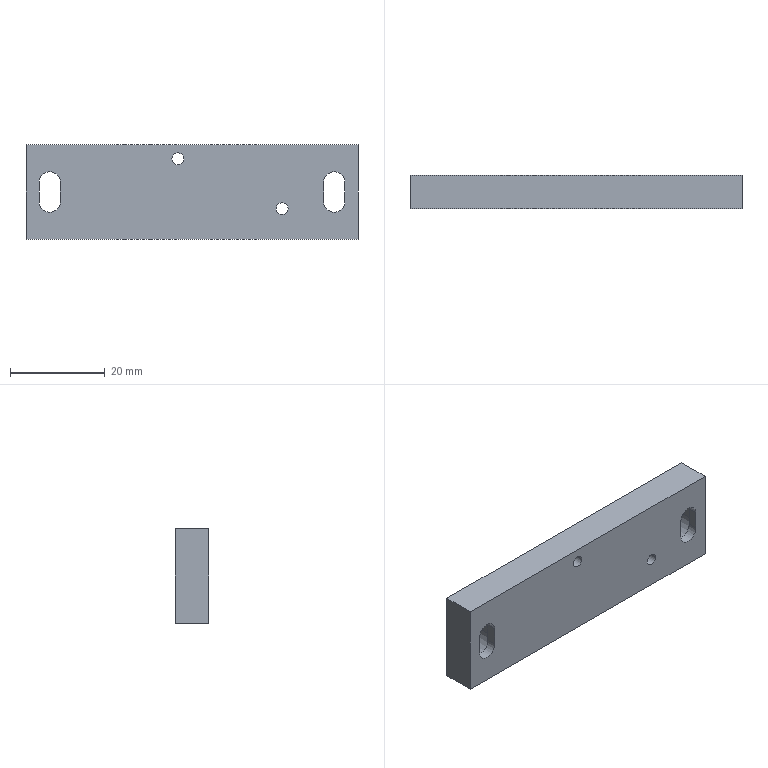Part | Creo | 1 solid | 32 faces | box 70 x 7 x 20 mm | volume 8772 mm3 | plane 16 | cylinder 12 | cone 4 | commonest cylinder face diameters 2.5 x4 4.5 x4 8 x4
STEP:
#1=CARTESIAN_POINT('',(-13.75,343.995,-332.));
#2=VERTEX_POINT('',#1);
#3=CARTESIAN_POINT('',(-83.75,343.995,-332.));
#4=VERTEX_POINT('',#3);
#5=CARTESIAN_POINT('',(-13.75,343.995,-332.));
#6=DIRECTION('',(-1.,0.,0.));
#7=VECTOR('',#6,70.);
#8=LINE('',#5,#7);
#9=EDGE_CURVE('',#2,#4,#8,.T.);
#10=ORIENTED_EDGE('',*,*,#9,.F.);
#11=CARTESIAN_POINT('',(-13.75,343.995,-352.));
#12=VERTEX_POINT('',#11);
#13=CARTESIAN_POINT('',(-13.75,343.995,-352.));
#14=DIRECTION('',(0.,0.,1.));
#15=VECTOR('',#14,20.);
#16=LINE('',#13,#15);
#17=EDGE_CURVE('',#12,#2,#16,.T.);
#18=ORIENTED_EDGE('',*,*,#17,.F.);
#19=CARTESIAN_POINT('',(-83.75,343.995,-352.));
#20=VERTEX_POINT('',#19);
#21=CARTESIAN_POINT('',(-83.75,343.995,-352.));
#22=DIRECTION('',(1.,0.,0.));
#23=VECTOR('',#22,70.);
#24=LINE('',#21,#23);
#25=EDGE_CURVE('',#20,#12,#24,.T.);
#26=ORIENTED_EDGE('',*,*,#25,.F.);
#27=CARTESIAN_POINT('',(-83.75,343.995,-332.));
#28=DIRECTION('',(0.,0.,-1.));
#29=VECTOR('',#28,20.);
#30=LINE('',#27,#29);
#31=EDGE_CURVE('',#4,#20,#30,.T.);
#32=ORIENTED_EDGE('',*,*,#31,.F.);
#33=EDGE_LOOP('',(#10,#18,#26,#32));
#34=FACE_OUTER_BOUND('',#33,.F.);
#35=CARTESIAN_POINT('',(-16.5,343.995,-344.));
#36=VERTEX_POINT('',#35);
#37=CARTESIAN_POINT('',(-16.5,343.995,-340.));
#38=VERTEX_POINT('',#37);
#39=CARTESIAN_POINT('',(-16.5,343.995,-344.));
#40=DIRECTION('',(0.,0.,1.));
#41=VECTOR('',#40,4.);
#42=LINE('',#39,#41);
#43=EDGE_CURVE('',#36,#38,#42,.T.);
#44=ORIENTED_EDGE('',*,*,#43,.T.);
#45=CARTESIAN_POINT('',(-21.,343.995,-340.));
#46=VERTEX_POINT('',#45);
#47=CARTESIAN_POINT('',(-18.75,343.995,-340.));
#48=DIRECTION('',(0.,1.,0.));
#49=DIRECTION('',(-1.,0.,0.));
#50=AXIS2_PLACEMENT_3D('',#47,#48,#49);
#51=CIRCLE('',#50,2.25);
#52=EDGE_CURVE('',#46,#38,#51,.T.);
#53=ORIENTED_EDGE('',*,*,#52,.F.);
#54=CARTESIAN_POINT('',(-21.,343.995,-344.));
#55=VERTEX_POINT('',#54);
#56=CARTESIAN_POINT('',(-21.,343.995,-340.));
#57=DIRECTION('',(0.,0.,-1.));
#58=VECTOR('',#57,4.);
#59=LINE('',#56,#58);
#60=EDGE_CURVE('',#46,#55,#59,.T.);
#61=ORIENTED_EDGE('',*,*,#60,.T.);
#62=CARTESIAN_POINT('',(-18.75,343.995,-344.));
#63=DIRECTION('',(0.,1.,0.));
#64=DIRECTION('',(1.,0.,0.));
#65=AXIS2_PLACEMENT_3D('',#62,#63,#64);
#66=CIRCLE('',#65,2.25);
#67=EDGE_CURVE('',#36,#55,#66,.T.);
#68=ORIENTED_EDGE('',*,*,#67,.F.);
#69=EDGE_LOOP('',(#44,#53,#61,#68));
#70=FACE_BOUND('',#69,.F.);
#71=CARTESIAN_POINT('',(-76.5,343.995,-344.));
#72=VERTEX_POINT('',#71);
#73=CARTESIAN_POINT('',(-81.,343.995,-344.));
#74=VERTEX_POINT('',#73);
#75=CARTESIAN_POINT('',(-78.75,343.995,-344.));
#76=DIRECTION('',(0.,1.,0.));
#77=DIRECTION('',(1.,0.,0.));
#78=AXIS2_PLACEMENT_3D('',#75,#76,#77);
#79=CIRCLE('',#78,2.25);
#80=EDGE_CURVE('',#72,#74,#79,.T.);
#81=ORIENTED_EDGE('',*,*,#80,.F.);
#82=CARTESIAN_POINT('',(-76.5,343.995,-340.));
#83=VERTEX_POINT('',#82);
#84=CARTESIAN_POINT('',(-76.5,343.995,-344.));
#85=DIRECTION('',(0.,0.,1.));
#86=VECTOR('',#85,4.);
#87=LINE('',#84,#86);
#88=EDGE_CURVE('',#72,#83,#87,.T.);
#89=ORIENTED_EDGE('',*,*,#88,.T.);
#90=CARTESIAN_POINT('',(-81.,343.995,-340.));
#91=VERTEX_POINT('',#90);
#92=CARTESIAN_POINT('',(-78.75,343.995,-340.));
#93=DIRECTION('',(0.,1.,0.));
#94=DIRECTION('',(-1.,0.,0.));
#95=AXIS2_PLACEMENT_3D('',#92,#93,#94);
#96=CIRCLE('',#95,2.25);
#97=EDGE_CURVE('',#91,#83,#96,.T.);
#98=ORIENTED_EDGE('',*,*,#97,.F.);
#99=CARTESIAN_POINT('',(-81.,343.995,-340.));
#100=DIRECTION('',(0.,0.,-1.));
#101=VECTOR('',#100,4.);
#102=LINE('',#99,#101);
#103=EDGE_CURVE('',#91,#74,#102,.T.);
#104=ORIENTED_EDGE('',*,*,#103,.T.);
#105=EDGE_LOOP('',(#81,#89,#98,#104));
#106=FACE_BOUND('',#105,.F.);
#107=CARTESIAN_POINT('',(-53.,343.995,-335.));
#108=VERTEX_POINT('',#107);
#109=CARTESIAN_POINT('',(-50.5,343.995,-335.));
#110=VERTEX_POINT('',#109);
#111=CARTESIAN_POINT('',(-51.75,343.995,-335.));
#112=DIRECTION('',(0.,1.,0.));
#113=DIRECTION('',(-1.,0.,0.));
#114=AXIS2_PLACEMENT_3D('',#111,#112,#113);
#115=CIRCLE('',#114,1.25);
#116=EDGE_CURVE('',#108,#110,#115,.T.);
#117=ORIENTED_EDGE('',*,*,#116,.F.);
#118=CARTESIAN_POINT('',(-51.75,343.995,-335.));
#119=DIRECTION('',(0.,1.,0.));
#120=DIRECTION('',(1.,0.,0.));
#121=AXIS2_PLACEMENT_3D('',#118,#119,#120);
#122=CIRCLE('',#121,1.25);
#123=EDGE_CURVE('',#110,#108,#122,.T.);
#124=ORIENTED_EDGE('',*,*,#123,.F.);
#125=EDGE_LOOP('',(#117,#124));
#126=FACE_BOUND('',#125,.F.);
#127=CARTESIAN_POINT('',(-31.,343.995,-345.5));
#128=VERTEX_POINT('',#127);
#129=CARTESIAN_POINT('',(-28.5,343.995,-345.5));
#130=VERTEX_POINT('',#129);
#131=CARTESIAN_POINT('',(-29.75,343.995,-345.5));
#132=DIRECTION('',(0.,1.,0.));
#133=DIRECTION('',(-1.,0.,0.));
#134=AXIS2_PLACEMENT_3D('',#131,#132,#133);
#135=CIRCLE('',#134,1.25);
#136=EDGE_CURVE('',#128,#130,#135,.T.);
#137=ORIENTED_EDGE('',*,*,#136,.F.);
#138=CARTESIAN_POINT('',(-29.75,343.995,-345.5));
#139=DIRECTION('',(0.,1.,0.));
#140=DIRECTION('',(1.,0.,0.));
#141=AXIS2_PLACEMENT_3D('',#138,#139,#140);
#142=CIRCLE('',#141,1.25);
#143=EDGE_CURVE('',#130,#128,#142,.T.);
#144=ORIENTED_EDGE('',*,*,#143,.F.);
#145=EDGE_LOOP('',(#137,#144));
#146=FACE_BOUND('',#145,.F.);
#147=CARTESIAN_POINT('',(-48.75,343.995,-342.));
#148=DIRECTION('',(0.,1.,0.));
#149=DIRECTION('',(1.,0.,0.));
#150=AXIS2_PLACEMENT_3D('',#147,#148,#149);
#151=PLANE('',#150);
#152=ADVANCED_FACE('',(#34,#70,#106,#126,#146),#151,.F.);
#153=CARTESIAN_POINT('',(-13.75,350.995,-332.));
#154=VERTEX_POINT('',#153);
#155=CARTESIAN_POINT('',(-13.75,350.995,-332.));
#156=DIRECTION('',(0.,-1.,0.));
#157=VECTOR('',#156,7.);
#158=LINE('',#155,#157);
#159=EDGE_CURVE('',#154,#2,#158,.T.);
#160=ORIENTED_EDGE('',*,*,#159,.T.);
#161=ORIENTED_EDGE('',*,*,#9,.T.);
#162=CARTESIAN_POINT('',(-83.75,350.995,-332.));
#163=VERTEX_POINT('',#162);
#164=CARTESIAN_POINT('',(-83.75,350.995,-332.));
#165=DIRECTION('',(0.,-1.,0.));
#166=VECTOR('',#165,7.);
#167=LINE('',#164,#166);
#168=EDGE_CURVE('',#163,#4,#167,.T.);
#169=ORIENTED_EDGE('',*,*,#168,.F.);
#170=CARTESIAN_POINT('',(-13.75,350.995,-332.));
#171=DIRECTION('',(-1.,0.,0.));
#172=VECTOR('',#171,70.);
#173=LINE('',#170,#172);
#174=EDGE_CURVE('',#154,#163,#173,.T.);
#175=ORIENTED_EDGE('',*,*,#174,.F.);
#176=EDGE_LOOP('',(#160,#161,#169,#175));
#177=FACE_OUTER_BOUND('',#176,.F.);
#178=CARTESIAN_POINT('',(-83.75,343.995,-332.));
#179=DIRECTION('',(0.,0.,1.));
#180=DIRECTION('',(-1.,0.,0.));
#181=AXIS2_PLACEMENT_3D('',#178,#179,#180);
#182=PLANE('',#181);
#183=ADVANCED_FACE('',(#177),#182,.T.);
#184=CARTESIAN_POINT('',(-13.75,350.995,-352.));
#185=VERTEX_POINT('',#184);
#186=CARTESIAN_POINT('',(-13.75,350.995,-352.));
#187=DIRECTION('',(0.,-1.,0.));
#188=VECTOR('',#187,7.);
#189=LINE('',#186,#188);
#190=EDGE_CURVE('',#185,#12,#189,.T.);
#191=ORIENTED_EDGE('',*,*,#190,.T.);
#192=ORIENTED_EDGE('',*,*,#17,.T.);
#193=ORIENTED_EDGE('',*,*,#159,.F.);
#194=CARTESIAN_POINT('',(-13.75,350.995,-352.));
#195=DIRECTION('',(0.,0.,1.));
#196=VECTOR('',#195,20.);
#197=LINE('',#194,#196);
#198=EDGE_CURVE('',#185,#154,#197,.T.);
#199=ORIENTED_EDGE('',*,*,#198,.F.);
#200=EDGE_LOOP('',(#191,#192,#193,#199));
#201=FACE_OUTER_BOUND('',#200,.F.);
#202=CARTESIAN_POINT('',(-13.75,343.995,-332.));
#203=DIRECTION('',(1.,0.,0.));
#204=DIRECTION('',(0.,0.,1.));
#205=AXIS2_PLACEMENT_3D('',#202,#203,#204);
#206=PLANE('',#205);
#207=ADVANCED_FACE('',(#201),#206,.T.);
#208=CARTESIAN_POINT('',(-83.75,350.995,-352.));
#209=VERTEX_POINT('',#208);
#210=CARTESIAN_POINT('',(-83.75,350.995,-352.));
#211=DIRECTION('',(0.,-1.,0.));
#212=VECTOR('',#211,7.);
#213=LINE('',#210,#212);
#214=EDGE_CURVE('',#209,#20,#213,.T.);
#215=ORIENTED_EDGE('',*,*,#214,.T.);
#216=ORIENTED_EDGE('',*,*,#25,.T.);
#217=ORIENTED_EDGE('',*,*,#190,.F.);
#218=CARTESIAN_POINT('',(-83.75,350.995,-352.));
#219=DIRECTION('',(1.,0.,0.));
#220=VECTOR('',#219,70.);
#221=LINE('',#218,#220);
#222=EDGE_CURVE('',#209,#185,#221,.T.);
#223=ORIENTED_EDGE('',*,*,#222,.F.);
#224=EDGE_LOOP('',(#215,#216,#217,#223));
#225=FACE_OUTER_BOUND('',#224,.F.);
#226=CARTESIAN_POINT('',(-13.75,343.995,-352.));
#227=DIRECTION('',(0.,0.,-1.));
#228=DIRECTION('',(1.,0.,0.));
#229=AXIS2_PLACEMENT_3D('',#226,#227,#228);
#230=PLANE('',#229);
#231=ADVANCED_FACE('',(#225),#230,.T.);
#232=ORIENTED_EDGE('',*,*,#168,.T.);
#233=ORIENTED_EDGE('',*,*,#31,.T.);
#234=ORIENTED_EDGE('',*,*,#214,.F.);
#235=CARTESIAN_POINT('',(-83.75,350.995,-332.));
#236=DIRECTION('',(0.,0.,-1.));
#237=VECTOR('',#236,20.);
#238=LINE('',#235,#237);
#239=EDGE_CURVE('',#163,#209,#238,.T.);
#240=ORIENTED_EDGE('',*,*,#239,.F.);
#241=EDGE_LOOP('',(#232,#233,#234,#240));
#242=FACE_OUTER_BOUND('',#241,.F.);
#243=CARTESIAN_POINT('',(-83.75,343.995,-352.));
#244=DIRECTION('',(-1.,0.,0.));
#245=DIRECTION('',(0.,0.,-1.));
#246=AXIS2_PLACEMENT_3D('',#243,#244,#245);
#247=PLANE('',#246);
#248=ADVANCED_FACE('',(#242),#247,.T.);
#249=ORIENTED_EDGE('',*,*,#222,.T.);
#250=ORIENTED_EDGE('',*,*,#198,.T.);
#251=ORIENTED_EDGE('',*,*,#174,.T.);
#252=ORIENTED_EDGE('',*,*,#239,.T.);
#253=EDGE_LOOP('',(#249,#250,#251,#252));
#254=FACE_OUTER_BOUND('',#253,.F.);
#255=CARTESIAN_POINT('',(-22.75,350.995,-340.));
#256=VERTEX_POINT('',#255);
#257=CARTESIAN_POINT('',(-22.75,350.995,-344.));
#258=VERTEX_POINT('',#257);
#259=CARTESIAN_POINT('',(-22.75,350.995,-340.));
#260=DIRECTION('',(0.,0.,-1.));
#261=VECTOR('',#260,4.);
#262=LINE('',#259,#261);
#263=EDGE_CURVE('',#256,#258,#262,.T.);
#264=ORIENTED_EDGE('',*,*,#263,.F.);
#265=CARTESIAN_POINT('',(-14.75,350.995,-340.));
#266=VERTEX_POINT('',#265);
#267=CARTESIAN_POINT('',(-18.75,350.995,-340.));
#268=DIRECTION('',(0.,-1.,0.));
#269=DIRECTION('',(1.,0.,0.));
#270=AXIS2_PLACEMENT_3D('',#267,#268,#269);
#271=CIRCLE('',#270,4.);
#272=EDGE_CURVE('',#266,#256,#271,.T.);
#273=ORIENTED_EDGE('',*,*,#272,.F.);
#274=CARTESIAN_POINT('',(-14.75,350.995,-344.));
#275=VERTEX_POINT('',#274);
#276=CARTESIAN_POINT('',(-14.75,350.995,-344.));
#277=DIRECTION('',(0.,0.,1.));
#278=VECTOR('',#277,4.);
#279=LINE('',#276,#278);
#280=EDGE_CURVE('',#275,#266,#279,.T.);
#281=ORIENTED_EDGE('',*,*,#280,.F.);
#282=CARTESIAN_POINT('',(-18.75,350.995,-344.));
#283=DIRECTION('',(0.,-1.,0.));
#284=DIRECTION('',(-1.,0.,0.));
#285=AXIS2_PLACEMENT_3D('',#282,#283,#284);
#286=CIRCLE('',#285,4.);
#287=EDGE_CURVE('',#258,#275,#286,.T.);
#288=ORIENTED_EDGE('',*,*,#287,.F.);
#289=EDGE_LOOP('',(#264,#273,#281,#288));
#290=FACE_BOUND('',#289,.F.);
#291=CARTESIAN_POINT('',(-74.75,350.995,-340.));
#292=VERTEX_POINT('',#291);
#293=CARTESIAN_POINT('',(-82.75,350.995,-340.));
#294=VERTEX_POINT('',#293);
#295=CARTESIAN_POINT('',(-78.75,350.995,-340.));
#296=DIRECTION('',(0.,-1.,0.));
#297=DIRECTION('',(1.,0.,0.));
#298=AXIS2_PLACEMENT_3D('',#295,#296,#297);
#299=CIRCLE('',#298,4.);
#300=EDGE_CURVE('',#292,#294,#299,.T.);
#301=ORIENTED_EDGE('',*,*,#300,.F.);
#302=CARTESIAN_POINT('',(-74.75,350.995,-344.));
#303=VERTEX_POINT('',#302);
#304=CARTESIAN_POINT('',(-74.75,350.995,-344.));
#305=DIRECTION('',(0.,0.,1.));
#306=VECTOR('',#305,4.);
#307=LINE('',#304,#306);
#308=EDGE_CURVE('',#303,#292,#307,.T.);
#309=ORIENTED_EDGE('',*,*,#308,.F.);
#310=CARTESIAN_POINT('',(-82.75,350.995,-344.));
#311=VERTEX_POINT('',#310);
#312=CARTESIAN_POINT('',(-78.75,350.995,-344.));
#313=DIRECTION('',(0.,-1.,0.));
#314=DIRECTION('',(-1.,0.,0.));
#315=AXIS2_PLACEMENT_3D('',#312,#313,#314);
#316=CIRCLE('',#315,4.);
#317=EDGE_CURVE('',#311,#303,#316,.T.);
#318=ORIENTED_EDGE('',*,*,#317,.F.);
#319=CARTESIAN_POINT('',(-82.75,350.995,-340.));
#320=DIRECTION('',(0.,0.,-1.));
#321=VECTOR('',#320,4.);
#322=LINE('',#319,#321);
#323=EDGE_CURVE('',#294,#311,#322,.T.);
#324=ORIENTED_EDGE('',*,*,#323,.F.);
#325=EDGE_LOOP('',(#301,#309,#318,#324));
#326=FACE_BOUND('',#325,.F.);
#327=CARTESIAN_POINT('',(-50.188,350.995,-335.));
#328=VERTEX_POINT('',#327);
#329=CARTESIAN_POINT('',(-53.312,350.995,-335.));
#330=VERTEX_POINT('',#329);
#331=CARTESIAN_POINT('',(-51.75,350.995,-335.));
#332=DIRECTION('',(0.,-1.,0.));
#333=DIRECTION('',(1.,0.,0.));
#334=AXIS2_PLACEMENT_3D('',#331,#332,#333);
#335=CIRCLE('',#334,1.562);
#336=EDGE_CURVE('',#328,#330,#335,.T.);
#337=ORIENTED_EDGE('',*,*,#336,.F.);
#338=CARTESIAN_POINT('',(-51.75,350.995,-335.));
#339=DIRECTION('',(0.,-1.,0.));
#340=DIRECTION('',(-1.,0.,0.));
#341=AXIS2_PLACEMENT_3D('',#338,#339,#340);
#342=CIRCLE('',#341,1.562);
#343=EDGE_CURVE('',#330,#328,#342,.T.);
#344=ORIENTED_EDGE('',*,*,#343,.F.);
#345=EDGE_LOOP('',(#337,#344));
#346=FACE_BOUND('',#345,.F.);
#347=CARTESIAN_POINT('',(-28.188,350.995,-345.5));
#348=VERTEX_POINT('',#347);
#349=CARTESIAN_POINT('',(-31.312,350.995,-345.5));
#350=VERTEX_POINT('',#349);
#351=CARTESIAN_POINT('',(-29.75,350.995,-345.5));
#352=DIRECTION('',(0.,-1.,0.));
#353=DIRECTION('',(1.,0.,0.));
#354=AXIS2_PLACEMENT_3D('',#351,#352,#353);
#355=CIRCLE('',#354,1.562);
#356=EDGE_CURVE('',#348,#350,#355,.T.);
#357=ORIENTED_EDGE('',*,*,#356,.F.);
#358=CARTESIAN_POINT('',(-29.75,350.995,-345.5));
#359=DIRECTION('',(0.,-1.,0.));
#360=DIRECTION('',(-1.,0.,0.));
#361=AXIS2_PLACEMENT_3D('',#358,#359,#360);
#362=CIRCLE('',#361,1.562);
#363=EDGE_CURVE('',#350,#348,#362,.T.);
#364=ORIENTED_EDGE('',*,*,#363,.F.);
#365=EDGE_LOOP('',(#357,#364));
#366=FACE_BOUND('',#365,.F.);
#367=CARTESIAN_POINT('',(-48.75,350.995,-342.));
#368=DIRECTION('',(0.,1.,0.));
#369=DIRECTION('',(1.,0.,0.));
#370=AXIS2_PLACEMENT_3D('',#367,#368,#369);
#371=PLANE('',#370);
#372=ADVANCED_FACE('',(#254,#290,#326,#346,#366),#371,.T.);
#373=CARTESIAN_POINT('',(-22.75,345.995,-340.));
#374=VERTEX_POINT('',#373);
#375=CARTESIAN_POINT('',(-22.75,345.995,-340.));
#376=DIRECTION('',(0.,1.,0.));
#377=VECTOR('',#376,5.);
#378=LINE('',#375,#377);
#379=EDGE_CURVE('',#374,#256,#378,.T.);
#380=ORIENTED_EDGE('',*,*,#379,.T.);
#381=ORIENTED_EDGE('',*,*,#263,.T.);
#382=CARTESIAN_POINT('',(-22.75,345.995,-344.));
#383=VERTEX_POINT('',#382);
#384=CARTESIAN_POINT('',(-22.75,350.995,-344.));
#385=DIRECTION('',(0.,-1.,0.));
#386=VECTOR('',#385,5.);
#387=LINE('',#384,#386);
#388=EDGE_CURVE('',#258,#383,#387,.T.);
#389=ORIENTED_EDGE('',*,*,#388,.T.);
#390=CARTESIAN_POINT('',(-22.75,345.995,-340.));
#391=DIRECTION('',(0.,0.,-1.));
#392=VECTOR('',#391,4.);
#393=LINE('',#390,#392);
#394=EDGE_CURVE('',#374,#383,#393,.T.);
#395=ORIENTED_EDGE('',*,*,#394,.F.);
#396=EDGE_LOOP('',(#380,#381,#389,#395));
#397=FACE_OUTER_BOUND('',#396,.F.);
#398=CARTESIAN_POINT('',(-22.75,350.995,-344.));
#399=DIRECTION('',(-1.,0.,0.));
#400=DIRECTION('',(0.,0.,-1.));
#401=AXIS2_PLACEMENT_3D('',#398,#399,#400);
#402=PLANE('',#401);
#403=ADVANCED_FACE('',(#397),#402,.F.);
#404=CARTESIAN_POINT('',(-14.75,345.995,-340.));
#405=VERTEX_POINT('',#404);
#406=CARTESIAN_POINT('',(-14.75,350.995,-340.));
#407=DIRECTION('',(0.,-1.,0.));
#408=VECTOR('',#407,5.);
#409=LINE('',#406,#408);
#410=EDGE_CURVE('',#266,#405,#409,.T.);
#411=ORIENTED_EDGE('',*,*,#410,.F.);
#412=ORIENTED_EDGE('',*,*,#272,.T.);
#413=ORIENTED_EDGE('',*,*,#379,.F.);
#414=CARTESIAN_POINT('',(-18.75,345.995,-340.));
#415=DIRECTION('',(0.,1.,0.));
#416=DIRECTION('',(-1.,0.,0.));
#417=AXIS2_PLACEMENT_3D('',#414,#415,#416);
#418=CIRCLE('',#417,4.);
#419=EDGE_CURVE('',#374,#405,#418,.T.);
#420=ORIENTED_EDGE('',*,*,#419,.T.);
#421=EDGE_LOOP('',(#411,#412,#413,#420));
#422=FACE_OUTER_BOUND('',#421,.F.);
#423=CARTESIAN_POINT('',(-18.75,350.995,-340.));
#424=DIRECTION('',(0.,1.,0.));
#425=DIRECTION('',(1.,0.,0.));
#426=AXIS2_PLACEMENT_3D('',#423,#424,#425);
#427=CYLINDRICAL_SURFACE('',#426,4.);
#428=ADVANCED_FACE('',(#422),#427,.F.);
#429=CARTESIAN_POINT('',(-14.75,345.995,-344.));
#430=VERTEX_POINT('',#429);
#431=CARTESIAN_POINT('',(-14.75,345.995,-344.));
#432=DIRECTION('',(0.,1.,0.));
#433=VECTOR('',#432,5.);
#434=LINE('',#431,#433);
#435=EDGE_CURVE('',#430,#275,#434,.T.);
#436=ORIENTED_EDGE('',*,*,#435,.T.);
#437=ORIENTED_EDGE('',*,*,#280,.T.);
#438=ORIENTED_EDGE('',*,*,#410,.T.);
#439=CARTESIAN_POINT('',(-14.75,345.995,-344.));
#440=DIRECTION('',(0.,0.,1.));
#441=VECTOR('',#440,4.);
#442=LINE('',#439,#441);
#443=EDGE_CURVE('',#430,#405,#442,.T.);
#444=ORIENTED_EDGE('',*,*,#443,.F.);
#445=EDGE_LOOP('',(#436,#437,#438,#444));
#446=FACE_OUTER_BOUND('',#445,.F.);
#447=CARTESIAN_POINT('',(-14.75,350.995,-340.));
#448=DIRECTION('',(1.,0.,0.));
#449=DIRECTION('',(0.,0.,1.));
#450=AXIS2_PLACEMENT_3D('',#447,#448,#449);
#451=PLANE('',#450);
#452=ADVANCED_FACE('',(#446),#451,.F.);
#453=ORIENTED_EDGE('',*,*,#388,.F.);
#454=ORIENTED_EDGE('',*,*,#287,.T.);
#455=ORIENTED_EDGE('',*,*,#435,.F.);
#456=CARTESIAN_POINT('',(-18.75,345.995,-344.));
#457=DIRECTION('',(0.,1.,0.));
#458=DIRECTION('',(1.,0.,0.));
#459=AXIS2_PLACEMENT_3D('',#456,#457,#458);
#460=CIRCLE('',#459,4.);
#461=EDGE_CURVE('',#430,#383,#460,.T.);
#462=ORIENTED_EDGE('',*,*,#461,.T.);
#463=EDGE_LOOP('',(#453,#454,#455,#462));
#464=FACE_OUTER_BOUND('',#463,.F.);
#465=CARTESIAN_POINT('',(-18.75,350.995,-344.));
#466=DIRECTION('',(0.,1.,0.));
#467=DIRECTION('',(1.,0.,0.));
#468=AXIS2_PLACEMENT_3D('',#465,#466,#467);
#469=CYLINDRICAL_SURFACE('',#468,4.);
#470=ADVANCED_FACE('',(#464),#469,.F.);
#471=ORIENTED_EDGE('',*,*,#419,.F.);
#472=ORIENTED_EDGE('',*,*,#394,.T.);
#473=ORIENTED_EDGE('',*,*,#461,.F.);
#474=ORIENTED_EDGE('',*,*,#443,.T.);
#475=EDGE_LOOP('',(#471,#472,#473,#474));
#476=FACE_OUTER_BOUND('',#475,.F.);
#477=CARTESIAN_POINT('',(-16.5,345.995,-344.));
#478=VERTEX_POINT('',#477);
#479=CARTESIAN_POINT('',(-16.5,345.995,-340.));
#480=VERTEX_POINT('',#479);
#481=CARTESIAN_POINT('',(-16.5,345.995,-344.));
#482=DIRECTION('',(0.,0.,1.));
#483=VECTOR('',#482,4.);
#484=LINE('',#481,#483);
#485=EDGE_CURVE('',#478,#480,#484,.T.);
#486=ORIENTED_EDGE('',*,*,#485,.F.);
#487=CARTESIAN_POINT('',(-21.,345.995,-344.));
#488=VERTEX_POINT('',#487);
#489=CARTESIAN_POINT('',(-18.75,345.995,-344.));
#490=DIRECTION('',(0.,-1.,0.));
#491=DIRECTION('',(-1.,0.,0.));
#492=AXIS2_PLACEMENT_3D('',#489,#490,#491);
#493=CIRCLE('',#492,2.25);
#494=EDGE_CURVE('',#488,#478,#493,.T.);
#495=ORIENTED_EDGE('',*,*,#494,.F.);
#496=CARTESIAN_POINT('',(-21.,345.995,-340.));
#497=VERTEX_POINT('',#496);
#498=CARTESIAN_POINT('',(-21.,345.995,-340.));
#499=DIRECTION('',(0.,0.,-1.));
#500=VECTOR('',#499,4.);
#501=LINE('',#498,#500);
#502=EDGE_CURVE('',#497,#488,#501,.T.);
#503=ORIENTED_EDGE('',*,*,#502,.F.);
#504=CARTESIAN_POINT('',(-18.75,345.995,-340.));
#505=DIRECTION('',(0.,-1.,0.));
#506=DIRECTION('',(1.,0.,0.));
#507=AXIS2_PLACEMENT_3D('',#504,#505,#506);
#508=CIRCLE('',#507,2.25);
#509=EDGE_CURVE('',#480,#497,#508,.T.);
#510=ORIENTED_EDGE('',*,*,#509,.F.);
#511=EDGE_LOOP('',(#486,#495,#503,#510));
#512=FACE_BOUND('',#511,.F.);
#513=CARTESIAN_POINT('',(-18.75,345.995,-344.));
#514=DIRECTION('',(0.,-1.,0.));
#515=DIRECTION('',(-1.,0.,0.));
#516=AXIS2_PLACEMENT_3D('',#513,#514,#515);
#517=PLANE('',#516);
#518=ADVANCED_FACE('',(#476,#512),#517,.F.);
#519=CARTESIAN_POINT('',(-16.5,345.995,-340.));
#520=DIRECTION('',(0.,-1.,0.));
#521=VECTOR('',#520,2.);
#522=LINE('',#519,#521);
#523=EDGE_CURVE('',#480,#38,#522,.T.);
#524=ORIENTED_EDGE('',*,*,#523,.T.);
#525=ORIENTED_EDGE('',*,*,#43,.F.);
#526=CARTESIAN_POINT('',(-16.5,343.995,-344.));
#527=DIRECTION('',(0.,1.,0.));
#528=VECTOR('',#527,2.);
#529=LINE('',#526,#528);
#530=EDGE_CURVE('',#36,#478,#529,.T.);
#531=ORIENTED_EDGE('',*,*,#530,.T.);
#532=ORIENTED_EDGE('',*,*,#485,.T.);
#533=EDGE_LOOP('',(#524,#525,#531,#532));
#534=FACE_OUTER_BOUND('',#533,.F.);
#535=CARTESIAN_POINT('',(-16.5,350.995,-340.));
#536=DIRECTION('',(1.,0.,0.));
#537=DIRECTION('',(0.,0.,1.));
#538=AXIS2_PLACEMENT_3D('',#535,#536,#537);
#539=PLANE('',#538);
#540=ADVANCED_FACE('',(#534),#539,.F.);
#541=CARTESIAN_POINT('',(-21.,343.995,-340.));
#542=DIRECTION('',(0.,1.,0.));
#543=VECTOR('',#542,2.);
#544=LINE('',#541,#543);
#545=EDGE_CURVE('',#46,#497,#544,.T.);
#546=ORIENTED_EDGE('',*,*,#545,.F.);
#547=ORIENTED_EDGE('',*,*,#52,.T.);
#548=ORIENTED_EDGE('',*,*,#523,.F.);
#549=ORIENTED_EDGE('',*,*,#509,.T.);
#550=EDGE_LOOP('',(#546,#547,#548,#549));
#551=FACE_OUTER_BOUND('',#550,.F.);
#552=CARTESIAN_POINT('',(-18.75,350.995,-340.));
#553=DIRECTION('',(0.,1.,0.));
#554=DIRECTION('',(1.,0.,0.));
#555=AXIS2_PLACEMENT_3D('',#552,#553,#554);
#556=CYLINDRICAL_SURFACE('',#555,2.25);
#557=ADVANCED_FACE('',(#551),#556,.F.);
#558=ORIENTED_EDGE('',*,*,#502,.T.);
#559=CARTESIAN_POINT('',(-21.,345.995,-344.));
#560=DIRECTION('',(0.,-1.,0.));
#561=VECTOR('',#560,2.);
#562=LINE('',#559,#561);
#563=EDGE_CURVE('',#488,#55,#562,.T.);
#564=ORIENTED_EDGE('',*,*,#563,.T.);
#565=ORIENTED_EDGE('',*,*,#60,.F.);
#566=ORIENTED_EDGE('',*,*,#545,.T.);
#567=EDGE_LOOP('',(#558,#564,#565,#566));
#568=FACE_OUTER_BOUND('',#567,.F.);
#569=CARTESIAN_POINT('',(-21.,350.995,-344.));
#570=DIRECTION('',(-1.,0.,0.));
#571=DIRECTION('',(0.,0.,-1.));
#572=AXIS2_PLACEMENT_3D('',#569,#570,#571);
#573=PLANE('',#572);
#574=ADVANCED_FACE('',(#568),#573,.F.);
#575=ORIENTED_EDGE('',*,*,#563,.F.);
#576=ORIENTED_EDGE('',*,*,#494,.T.);
#577=ORIENTED_EDGE('',*,*,#530,.F.);
#578=ORIENTED_EDGE('',*,*,#67,.T.);
#579=EDGE_LOOP('',(#575,#576,#577,#578));
#580=FACE_OUTER_BOUND('',#579,.F.);
#581=CARTESIAN_POINT('',(-18.75,350.995,-344.));
#582=DIRECTION('',(0.,1.,0.));
#583=DIRECTION('',(1.,0.,0.));
#584=AXIS2_PLACEMENT_3D('',#581,#582,#583);
#585=CYLINDRICAL_SURFACE('',#584,2.25);
#586=ADVANCED_FACE('',(#580),#585,.F.);
#587=CARTESIAN_POINT('',(-74.75,345.995,-340.));
#588=VERTEX_POINT('',#587);
#589=CARTESIAN_POINT('',(-74.75,350.995,-340.));
#590=DIRECTION('',(0.,-1.,0.));
#591=VECTOR('',#590,5.);
#592=LINE('',#589,#591);
#593=EDGE_CURVE('',#292,#588,#592,.T.);
#594=ORIENTED_EDGE('',*,*,#593,.F.);
#595=ORIENTED_EDGE('',*,*,#300,.T.);
#596=CARTESIAN_POINT('',(-82.75,345.995,-340.));
#597=VERTEX_POINT('',#596);
#598=CARTESIAN_POINT('',(-82.75,345.995,-340.));
#599=DIRECTION('',(0.,1.,0.));
#600=VECTOR('',#599,5.);
#601=LINE('',#598,#600);
#602=EDGE_CURVE('',#597,#294,#601,.T.);
#603=ORIENTED_EDGE('',*,*,#602,.F.);
#604=CARTESIAN_POINT('',(-78.75,345.995,-340.));
#605=DIRECTION('',(0.,1.,0.));
#606=DIRECTION('',(-1.,0.,0.));
#607=AXIS2_PLACEMENT_3D('',#604,#605,#606);
#608=CIRCLE('',#607,4.);
#609=EDGE_CURVE('',#597,#588,#608,.T.);
#610=ORIENTED_EDGE('',*,*,#609,.T.);
#611=EDGE_LOOP('',(#594,#595,#603,#610));
#612=FACE_OUTER_BOUND('',#611,.F.);
#613=CARTESIAN_POINT('',(-78.75,350.995,-340.));
#614=DIRECTION('',(0.,1.,0.));
#615=DIRECTION('',(1.,0.,0.));
#616=AXIS2_PLACEMENT_3D('',#613,#614,#615);
#617=CYLINDRICAL_SURFACE('',#616,4.);
#618=ADVANCED_FACE('',(#612),#617,.F.);
#619=CARTESIAN_POINT('',(-74.75,345.995,-344.));
#620=VERTEX_POINT('',#619);
#621=CARTESIAN_POINT('',(-74.75,345.995,-344.));
#622=DIRECTION('',(0.,1.,0.));
#623=VECTOR('',#622,5.);
#624=LINE('',#621,#623);
#625=EDGE_CURVE('',#620,#303,#624,.T.);
#626=ORIENTED_EDGE('',*,*,#625,.T.);
#627=ORIENTED_EDGE('',*,*,#308,.T.);
#628=ORIENTED_EDGE('',*,*,#593,.T.);
#629=CARTESIAN_POINT('',(-74.75,345.995,-344.));
#630=DIRECTION('',(0.,0.,1.));
#631=VECTOR('',#630,4.);
#632=LINE('',#629,#631);
#633=EDGE_CURVE('',#620,#588,#632,.T.);
#634=ORIENTED_EDGE('',*,*,#633,.F.);
#635=EDGE_LOOP('',(#626,#627,#628,#634));
#636=FACE_OUTER_BOUND('',#635,.F.);
#637=CARTESIAN_POINT('',(-74.75,350.995,-340.));
#638=DIRECTION('',(1.,0.,0.));
#639=DIRECTION('',(0.,0.,1.));
#640=AXIS2_PLACEMENT_3D('',#637,#638,#639);
#641=PLANE('',#640);
#642=ADVANCED_FACE('',(#636),#641,.F.);
#643=CARTESIAN_POINT('',(-82.75,345.995,-344.));
#644=VERTEX_POINT('',#643);
#645=CARTESIAN_POINT('',(-82.75,350.995,-344.));
#646=DIRECTION('',(0.,-1.,0.));
#647=VECTOR('',#646,5.);
#648=LINE('',#645,#647);
#649=EDGE_CURVE('',#311,#644,#648,.T.);
#650=ORIENTED_EDGE('',*,*,#649,.F.);
#651=ORIENTED_EDGE('',*,*,#317,.T.);
#652=ORIENTED_EDGE('',*,*,#625,.F.);
#653=CARTESIAN_POINT('',(-78.75,345.995,-344.));
#654=DIRECTION('',(0.,1.,0.));
#655=DIRECTION('',(1.,0.,0.));
#656=AXIS2_PLACEMENT_3D('',#653,#654,#655);
#657=CIRCLE('',#656,4.);
#658=EDGE_CURVE('',#620,#644,#657,.T.);
#659=ORIENTED_EDGE('',*,*,#658,.T.);
#660=EDGE_LOOP('',(#650,#651,#652,#659));
#661=FACE_OUTER_BOUND('',#660,.F.);
#662=CARTESIAN_POINT('',(-78.75,350.995,-344.));
#663=DIRECTION('',(0.,1.,0.));
#664=DIRECTION('',(1.,0.,0.));
#665=AXIS2_PLACEMENT_3D('',#662,#663,#664);
#666=CYLINDRICAL_SURFACE('',#665,4.);
#667=ADVANCED_FACE('',(#661),#666,.F.);
#668=ORIENTED_EDGE('',*,*,#602,.T.);
#669=ORIENTED_EDGE('',*,*,#323,.T.);
#670=ORIENTED_EDGE('',*,*,#649,.T.);
#671=CARTESIAN_POINT('',(-82.75,345.995,-340.));
#672=DIRECTION('',(0.,0.,-1.));
#673=VECTOR('',#672,4.);
#674=LINE('',#671,#673);
#675=EDGE_CURVE('',#597,#644,#674,.T.);
#676=ORIENTED_EDGE('',*,*,#675,.F.);
#677=EDGE_LOOP('',(#668,#669,#670,#676));
#678=FACE_OUTER_BOUND('',#677,.F.);
#679=CARTESIAN_POINT('',(-82.75,350.995,-344.));
#680=DIRECTION('',(-1.,0.,0.));
#681=DIRECTION('',(0.,0.,-1.));
#682=AXIS2_PLACEMENT_3D('',#679,#680,#681);
#683=PLANE('',#682);
#684=ADVANCED_FACE('',(#678),#683,.F.);
#685=ORIENTED_EDGE('',*,*,#609,.F.);
#686=ORIENTED_EDGE('',*,*,#675,.T.);
#687=ORIENTED_EDGE('',*,*,#658,.F.);
#688=ORIENTED_EDGE('',*,*,#633,.T.);
#689=EDGE_LOOP('',(#685,#686,#687,#688));
#690=FACE_OUTER_BOUND('',#689,.F.);
#691=CARTESIAN_POINT('',(-76.5,345.995,-344.));
#692=VERTEX_POINT('',#691);
#693=CARTESIAN_POINT('',(-76.5,345.995,-340.));
#694=VERTEX_POINT('',#693);
#695=CARTESIAN_POINT('',(-76.5,345.995,-344.));
#696=DIRECTION('',(0.,0.,1.));
#697=VECTOR('',#696,4.);
#698=LINE('',#695,#697);
#699=EDGE_CURVE('',#692,#694,#698,.T.);
#700=ORIENTED_EDGE('',*,*,#699,.F.);
#701=CARTESIAN_POINT('',(-81.,345.995,-344.));
#702=VERTEX_POINT('',#701);
#703=CARTESIAN_POINT('',(-78.75,345.995,-344.));
#704=DIRECTION('',(0.,-1.,0.));
#705=DIRECTION('',(-1.,0.,0.));
#706=AXIS2_PLACEMENT_3D('',#703,#704,#705);
#707=CIRCLE('',#706,2.25);
#708=EDGE_CURVE('',#702,#692,#707,.T.);
#709=ORIENTED_EDGE('',*,*,#708,.F.);
#710=CARTESIAN_POINT('',(-81.,345.995,-340.));
#711=VERTEX_POINT('',#710);
#712=CARTESIAN_POINT('',(-81.,345.995,-340.));
#713=DIRECTION('',(0.,0.,-1.));
#714=VECTOR('',#713,4.);
#715=LINE('',#712,#714);
#716=EDGE_CURVE('',#711,#702,#715,.T.);
#717=ORIENTED_EDGE('',*,*,#716,.F.);
#718=CARTESIAN_POINT('',(-78.75,345.995,-340.));
#719=DIRECTION('',(0.,-1.,0.));
#720=DIRECTION('',(1.,0.,0.));
#721=AXIS2_PLACEMENT_3D('',#718,#719,#720);
#722=CIRCLE('',#721,2.25);
#723=EDGE_CURVE('',#694,#711,#722,.T.);
#724=ORIENTED_EDGE('',*,*,#723,.F.);
#725=EDGE_LOOP('',(#700,#709,#717,#724));
#726=FACE_BOUND('',#725,.F.);
#727=CARTESIAN_POINT('',(-78.75,345.995,-344.));
#728=DIRECTION('',(0.,-1.,0.));
#729=DIRECTION('',(-1.,0.,0.));
#730=AXIS2_PLACEMENT_3D('',#727,#728,#729);
#731=PLANE('',#730);
#732=ADVANCED_FACE('',(#690,#726),#731,.F.);
#733=CARTESIAN_POINT('',(-76.5,345.995,-340.));
#734=DIRECTION('',(0.,-1.,0.));
#735=VECTOR('',#734,2.);
#736=LINE('',#733,#735);
#737=EDGE_CURVE('',#694,#83,#736,.T.);
#738=ORIENTED_EDGE('',*,*,#737,.T.);
#739=ORIENTED_EDGE('',*,*,#88,.F.);
#740=CARTESIAN_POINT('',(-76.5,343.995,-344.));
#741=DIRECTION('',(0.,1.,0.));
#742=VECTOR('',#741,2.);
#743=LINE('',#740,#742);
#744=EDGE_CURVE('',#72,#692,#743,.T.);
#745=ORIENTED_EDGE('',*,*,#744,.T.);
#746=ORIENTED_EDGE('',*,*,#699,.T.);
#747=EDGE_LOOP('',(#738,#739,#745,#746));
#748=FACE_OUTER_BOUND('',#747,.F.);
#749=CARTESIAN_POINT('',(-76.5,350.995,-340.));
#750=DIRECTION('',(1.,0.,0.));
#751=DIRECTION('',(0.,0.,1.));
#752=AXIS2_PLACEMENT_3D('',#749,#750,#751);
#753=PLANE('',#752);
#754=ADVANCED_FACE('',(#748),#753,.F.);
#755=CARTESIAN_POINT('',(-81.,343.995,-340.));
#756=DIRECTION('',(0.,1.,0.));
#757=VECTOR('',#756,2.);
#758=LINE('',#755,#757);
#759=EDGE_CURVE('',#91,#711,#758,.T.);
#760=ORIENTED_EDGE('',*,*,#759,.F.);
#761=ORIENTED_EDGE('',*,*,#97,.T.);
#762=ORIENTED_EDGE('',*,*,#737,.F.);
#763=ORIENTED_EDGE('',*,*,#723,.T.);
#764=EDGE_LOOP('',(#760,#761,#762,#763));
#765=FACE_OUTER_BOUND('',#764,.F.);
#766=CARTESIAN_POINT('',(-78.75,350.995,-340.));
#767=DIRECTION('',(0.,1.,0.));
#768=DIRECTION('',(1.,0.,0.));
#769=AXIS2_PLACEMENT_3D('',#766,#767,#768);
#770=CYLINDRICAL_SURFACE('',#769,2.25);
#771=ADVANCED_FACE('',(#765),#770,.F.);
#772=ORIENTED_EDGE('',*,*,#716,.T.);
#773=CARTESIAN_POINT('',(-81.,345.995,-344.));
#774=DIRECTION('',(0.,-1.,0.));
#775=VECTOR('',#774,2.);
#776=LINE('',#773,#775);
#777=EDGE_CURVE('',#702,#74,#776,.T.);
#778=ORIENTED_EDGE('',*,*,#777,.T.);
#779=ORIENTED_EDGE('',*,*,#103,.F.);
#780=ORIENTED_EDGE('',*,*,#759,.T.);
#781=EDGE_LOOP('',(#772,#778,#779,#780));
#782=FACE_OUTER_BOUND('',#781,.F.);
#783=CARTESIAN_POINT('',(-81.,350.995,-344.));
#784=DIRECTION('',(-1.,0.,0.));
#785=DIRECTION('',(0.,0.,-1.));
#786=AXIS2_PLACEMENT_3D('',#783,#784,#785);
#787=PLANE('',#786);
#788=ADVANCED_FACE('',(#782),#787,.F.);
#789=ORIENTED_EDGE('',*,*,#777,.F.);
#790=ORIENTED_EDGE('',*,*,#708,.T.);
#791=ORIENTED_EDGE('',*,*,#744,.F.);
#792=ORIENTED_EDGE('',*,*,#80,.T.);
#793=EDGE_LOOP('',(#789,#790,#791,#792));
#794=FACE_OUTER_BOUND('',#793,.F.);
#795=CARTESIAN_POINT('',(-78.75,350.995,-344.));
#796=DIRECTION('',(0.,1.,0.));
#797=DIRECTION('',(1.,0.,0.));
#798=AXIS2_PLACEMENT_3D('',#795,#796,#797);
#799=CYLINDRICAL_SURFACE('',#798,2.25);
#800=ADVANCED_FACE('',(#794),#799,.F.);
#801=CARTESIAN_POINT('',(-50.5,350.683,-335.));
#802=VERTEX_POINT('',#801);
#803=CARTESIAN_POINT('',(-50.5,350.683,-335.));
#804=DIRECTION('',(0.7071,0.7071,0.));
#805=VECTOR('',#804,0.4419);
#806=LINE('',#803,#805);
#807=EDGE_CURVE('',#802,#328,#806,.T.);
#808=ORIENTED_EDGE('',*,*,#807,.T.);
#809=ORIENTED_EDGE('',*,*,#336,.T.);
#810=CARTESIAN_POINT('',(-53.,350.683,-335.));
#811=VERTEX_POINT('',#810);
#812=CARTESIAN_POINT('',(-53.312,350.995,-335.));
#813=DIRECTION('',(0.7071,-0.7071,0.));
#814=VECTOR('',#813,0.4419);
#815=LINE('',#812,#814);
#816=EDGE_CURVE('',#330,#811,#815,.T.);
#817=ORIENTED_EDGE('',*,*,#816,.T.);
#818=CARTESIAN_POINT('',(-51.75,350.683,-335.));
#819=DIRECTION('',(0.,-1.,0.));
#820=DIRECTION('',(1.,0.,0.));
#821=AXIS2_PLACEMENT_3D('',#818,#819,#820);
#822=CIRCLE('',#821,1.25);
#823=EDGE_CURVE('',#802,#811,#822,.T.);
#824=ORIENTED_EDGE('',*,*,#823,.F.);
#825=EDGE_LOOP('',(#808,#809,#817,#824));
#826=FACE_OUTER_BOUND('',#825,.F.);
#827=CARTESIAN_POINT('',(-51.75,350.839,-335.));
#828=DIRECTION('',(0.,1.,0.));
#829=DIRECTION('',(-1.,0.,0.));
#830=AXIS2_PLACEMENT_3D('',#827,#828,#829);
#831=CONICAL_SURFACE('',#830,1.406,45.);
#832=ADVANCED_FACE('',(#826),#831,.F.);
#833=ORIENTED_EDGE('',*,*,#816,.F.);
#834=ORIENTED_EDGE('',*,*,#343,.T.);
#835=ORIENTED_EDGE('',*,*,#807,.F.);
#836=CARTESIAN_POINT('',(-51.75,350.683,-335.));
#837=DIRECTION('',(0.,-1.,0.));
#838=DIRECTION('',(-1.,0.,0.));
#839=AXIS2_PLACEMENT_3D('',#836,#837,#838);
#840=CIRCLE('',#839,1.25);
#841=EDGE_CURVE('',#811,#802,#840,.T.);
#842=ORIENTED_EDGE('',*,*,#841,.F.);
#843=EDGE_LOOP('',(#833,#834,#835,#842));
#844=FACE_OUTER_BOUND('',#843,.F.);
#845=CARTESIAN_POINT('',(-51.75,350.839,-335.));
#846=DIRECTION('',(0.,1.,0.));
#847=DIRECTION('',(-1.,0.,0.));
#848=AXIS2_PLACEMENT_3D('',#845,#846,#847);
#849=CONICAL_SURFACE('',#848,1.406,45.);
#850=ADVANCED_FACE('',(#844),#849,.F.);
#851=CARTESIAN_POINT('',(-50.5,350.683,-335.));
#852=DIRECTION('',(0.,-1.,0.));
#853=VECTOR('',#852,6.688);
#854=LINE('',#851,#853);
#855=EDGE_CURVE('',#802,#110,#854,.T.);
#856=ORIENTED_EDGE('',*,*,#855,.T.);
#857=ORIENTED_EDGE('',*,*,#123,.T.);
#858=CARTESIAN_POINT('',(-53.,343.995,-335.));
#859=DIRECTION('',(0.,1.,0.));
#860=VECTOR('',#859,6.688);
#861=LINE('',#858,#860);
#862=EDGE_CURVE('',#108,#811,#861,.T.);
#863=ORIENTED_EDGE('',*,*,#862,.T.);
#864=ORIENTED_EDGE('',*,*,#841,.T.);
#865=EDGE_LOOP('',(#856,#857,#863,#864));
#866=FACE_OUTER_BOUND('',#865,.F.);
#867=CARTESIAN_POINT('',(-51.75,342.857,-335.));
#868=DIRECTION('',(0.,1.,0.));
#869=DIRECTION('',(-1.,0.,0.));
#870=AXIS2_PLACEMENT_3D('',#867,#868,#869);
#871=CYLINDRICAL_SURFACE('',#870,1.25);
#872=ADVANCED_FACE('',(#866),#871,.F.);
#873=ORIENTED_EDGE('',*,*,#862,.F.);
#874=ORIENTED_EDGE('',*,*,#116,.T.);
#875=ORIENTED_EDGE('',*,*,#855,.F.);
#876=ORIENTED_EDGE('',*,*,#823,.T.);
#877=EDGE_LOOP('',(#873,#874,#875,#876));
#878=FACE_OUTER_BOUND('',#877,.F.);
#879=CARTESIAN_POINT('',(-51.75,342.857,-335.));
#880=DIRECTION('',(0.,1.,0.));
#881=DIRECTION('',(-1.,0.,0.));
#882=AXIS2_PLACEMENT_3D('',#879,#880,#881);
#883=CYLINDRICAL_SURFACE('',#882,1.25);
#884=ADVANCED_FACE('',(#878),#883,.F.);
#885=CARTESIAN_POINT('',(-28.5,350.683,-345.5));
#886=VERTEX_POINT('',#885);
#887=CARTESIAN_POINT('',(-28.5,350.683,-345.5));
#888=DIRECTION('',(0.7071,0.7071,0.));
#889=VECTOR('',#888,0.4419);
#890=LINE('',#887,#889);
#891=EDGE_CURVE('',#886,#348,#890,.T.);
#892=ORIENTED_EDGE('',*,*,#891,.T.);
#893=ORIENTED_EDGE('',*,*,#356,.T.);
#894=CARTESIAN_POINT('',(-31.,350.683,-345.5));
#895=VERTEX_POINT('',#894);
#896=CARTESIAN_POINT('',(-31.312,350.995,-345.5));
#897=DIRECTION('',(0.7071,-0.7071,0.));
#898=VECTOR('',#897,0.4419);
#899=LINE('',#896,#898);
#900=EDGE_CURVE('',#350,#895,#899,.T.);
#901=ORIENTED_EDGE('',*,*,#900,.T.);
#902=CARTESIAN_POINT('',(-29.75,350.683,-345.5));
#903=DIRECTION('',(0.,-1.,0.));
#904=DIRECTION('',(1.,0.,0.));
#905=AXIS2_PLACEMENT_3D('',#902,#903,#904);
#906=CIRCLE('',#905,1.25);
#907=EDGE_CURVE('',#886,#895,#906,.T.);
#908=ORIENTED_EDGE('',*,*,#907,.F.);
#909=EDGE_LOOP('',(#892,#893,#901,#908));
#910=FACE_OUTER_BOUND('',#909,.F.);
#911=CARTESIAN_POINT('',(-29.75,350.839,-345.5));
#912=DIRECTION('',(0.,1.,0.));
#913=DIRECTION('',(-1.,0.,0.));
#914=AXIS2_PLACEMENT_3D('',#911,#912,#913);
#915=CONICAL_SURFACE('',#914,1.406,45.);
#916=ADVANCED_FACE('',(#910),#915,.F.);
#917=ORIENTED_EDGE('',*,*,#900,.F.);
#918=ORIENTED_EDGE('',*,*,#363,.T.);
#919=ORIENTED_EDGE('',*,*,#891,.F.);
#920=CARTESIAN_POINT('',(-29.75,350.683,-345.5));
#921=DIRECTION('',(0.,-1.,0.));
#922=DIRECTION('',(-1.,0.,0.));
#923=AXIS2_PLACEMENT_3D('',#920,#921,#922);
#924=CIRCLE('',#923,1.25);
#925=EDGE_CURVE('',#895,#886,#924,.T.);
#926=ORIENTED_EDGE('',*,*,#925,.F.);
#927=EDGE_LOOP('',(#917,#918,#919,#926));
#928=FACE_OUTER_BOUND('',#927,.F.);
#929=CARTESIAN_POINT('',(-29.75,350.839,-345.5));
#930=DIRECTION('',(0.,1.,0.));
#931=DIRECTION('',(-1.,0.,0.));
#932=AXIS2_PLACEMENT_3D('',#929,#930,#931);
#933=CONICAL_SURFACE('',#932,1.406,45.);
#934=ADVANCED_FACE('',(#928),#933,.F.);
#935=CARTESIAN_POINT('',(-28.5,350.683,-345.5));
#936=DIRECTION('',(0.,-1.,0.));
#937=VECTOR('',#936,6.688);
#938=LINE('',#935,#937);
#939=EDGE_CURVE('',#886,#130,#938,.T.);
#940=ORIENTED_EDGE('',*,*,#939,.T.);
#941=ORIENTED_EDGE('',*,*,#143,.T.);
#942=CARTESIAN_POINT('',(-31.,343.995,-345.5));
#943=DIRECTION('',(0.,1.,0.));
#944=VECTOR('',#943,6.688);
#945=LINE('',#942,#944);
#946=EDGE_CURVE('',#128,#895,#945,.T.);
#947=ORIENTED_EDGE('',*,*,#946,.T.);
#948=ORIENTED_EDGE('',*,*,#925,.T.);
#949=EDGE_LOOP('',(#940,#941,#947,#948));
#950=FACE_OUTER_BOUND('',#949,.F.);
#951=CARTESIAN_POINT('',(-29.75,342.857,-345.5));
#952=DIRECTION('',(0.,1.,0.));
#953=DIRECTION('',(-1.,0.,0.));
#954=AXIS2_PLACEMENT_3D('',#951,#952,#953);
#955=CYLINDRICAL_SURFACE('',#954,1.25);
#956=ADVANCED_FACE('',(#950),#955,.F.);
#957=ORIENTED_EDGE('',*,*,#946,.F.);
#958=ORIENTED_EDGE('',*,*,#136,.T.);
#959=ORIENTED_EDGE('',*,*,#939,.F.);
#960=ORIENTED_EDGE('',*,*,#907,.T.);
#961=EDGE_LOOP('',(#957,#958,#959,#960));
#962=FACE_OUTER_BOUND('',#961,.F.);
#963=CARTESIAN_POINT('',(-29.75,342.857,-345.5));
#964=DIRECTION('',(0.,1.,0.));
#965=DIRECTION('',(-1.,0.,0.));
#966=AXIS2_PLACEMENT_3D('',#963,#964,#965);
#967=CYLINDRICAL_SURFACE('',#966,1.25);
#968=ADVANCED_FACE('',(#962),#967,.F.);
#969=CLOSED_SHELL('',(#152,#183,#207,#231,#248,#372,#403,#428,#452,#470,#518,#540,#557,#574,#586,#618,#642,#667,#684,#732,#754,#771,#788,#800,#832,#850,#872,#884,#916,#934,#956,#968));
#970=MANIFOLD_SOLID_BREP('',#969);
#971=(LENGTH_UNIT()NAMED_UNIT(*)SI_UNIT(.MILLI.,.METRE.));
#972=UNCERTAINTY_MEASURE_WITH_UNIT(LENGTH_MEASURE(0.007313),#971,'','');
#973=(NAMED_UNIT(*)PLANE_ANGLE_UNIT()SI_UNIT($,.RADIAN.));
#974=PLANE_ANGLE_MEASURE_WITH_UNIT(PLANE_ANGLE_MEASURE(0.01745),#973);
#975=(CONVERSION_BASED_UNIT('DEGREE',#974)NAMED_UNIT(*)PLANE_ANGLE_UNIT());
#976=(NAMED_UNIT(*)SI_UNIT($,.STERADIAN.)SOLID_ANGLE_UNIT());
#977=(GEOMETRIC_REPRESENTATION_CONTEXT(3)GLOBAL_UNCERTAINTY_ASSIGNED_CONTEXT((#972))GLOBAL_UNIT_ASSIGNED_CONTEXT((#971,#975,#976))REPRESENTATION_CONTEXT('',''));
#978=ADVANCED_BREP_SHAPE_REPRESENTATION('',(#970),#977);